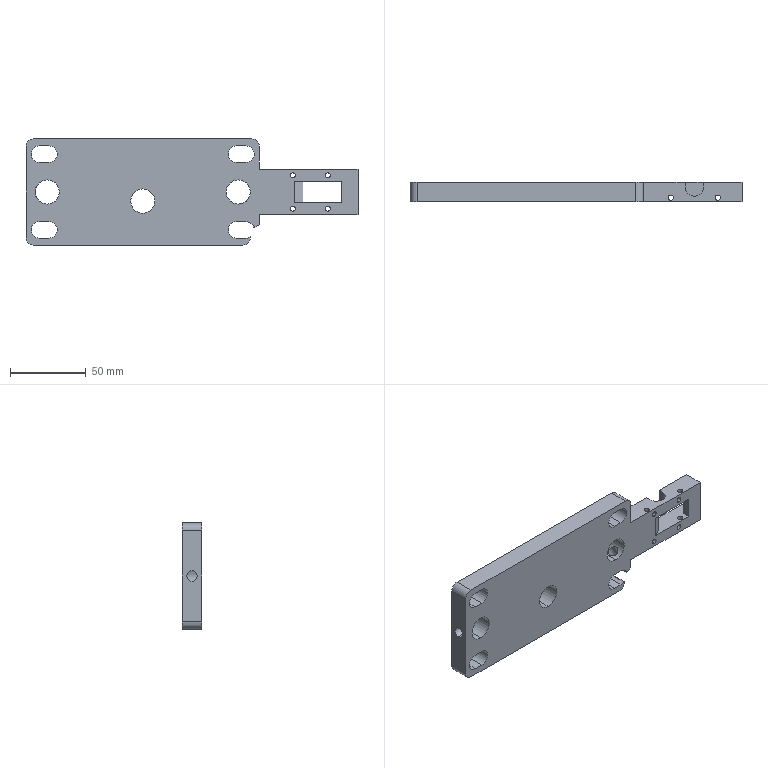Part | 1 solid | 67 faces | box 219 x 13 x 70 mm | volume 140001 mm3 | cylinder 39 | plane 28 | commonest cylinder face diameters 11 x9 3.3 x8 3.5 x6 16 x6 6.8 x4 10 x4